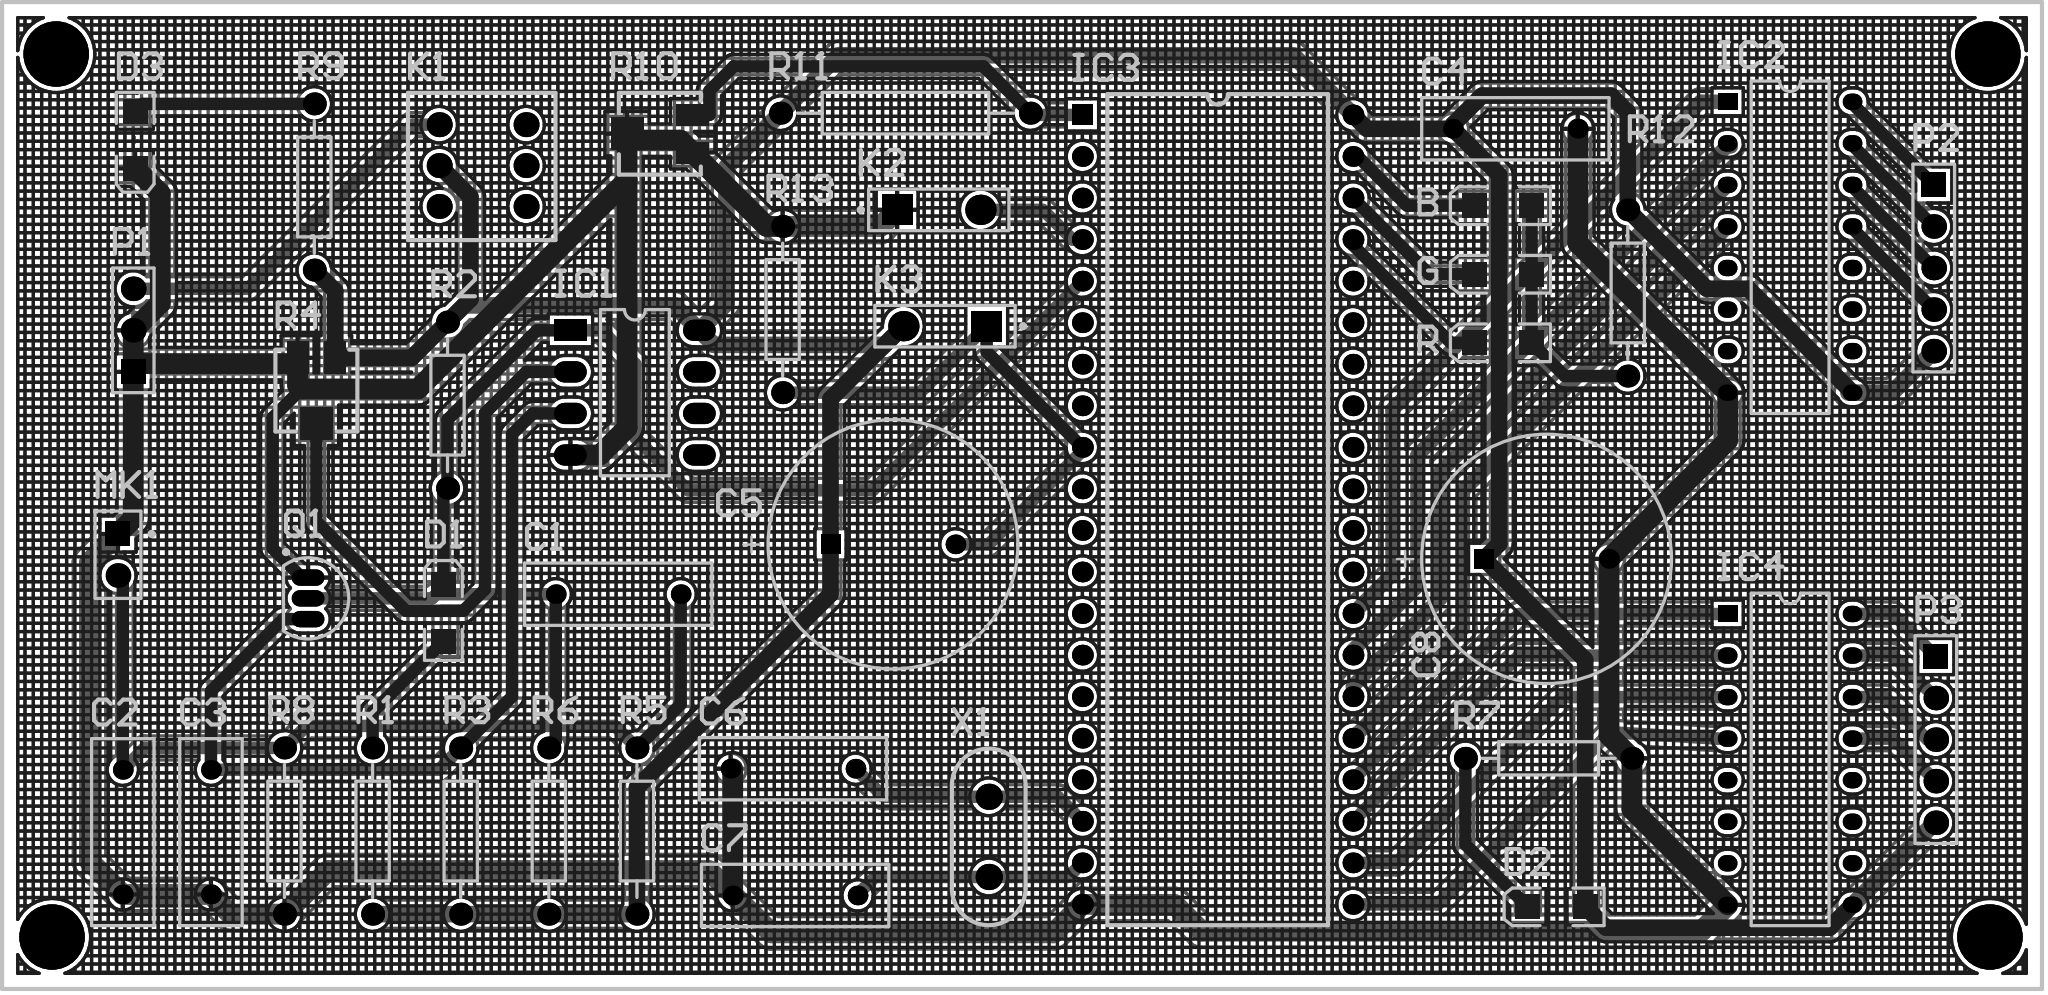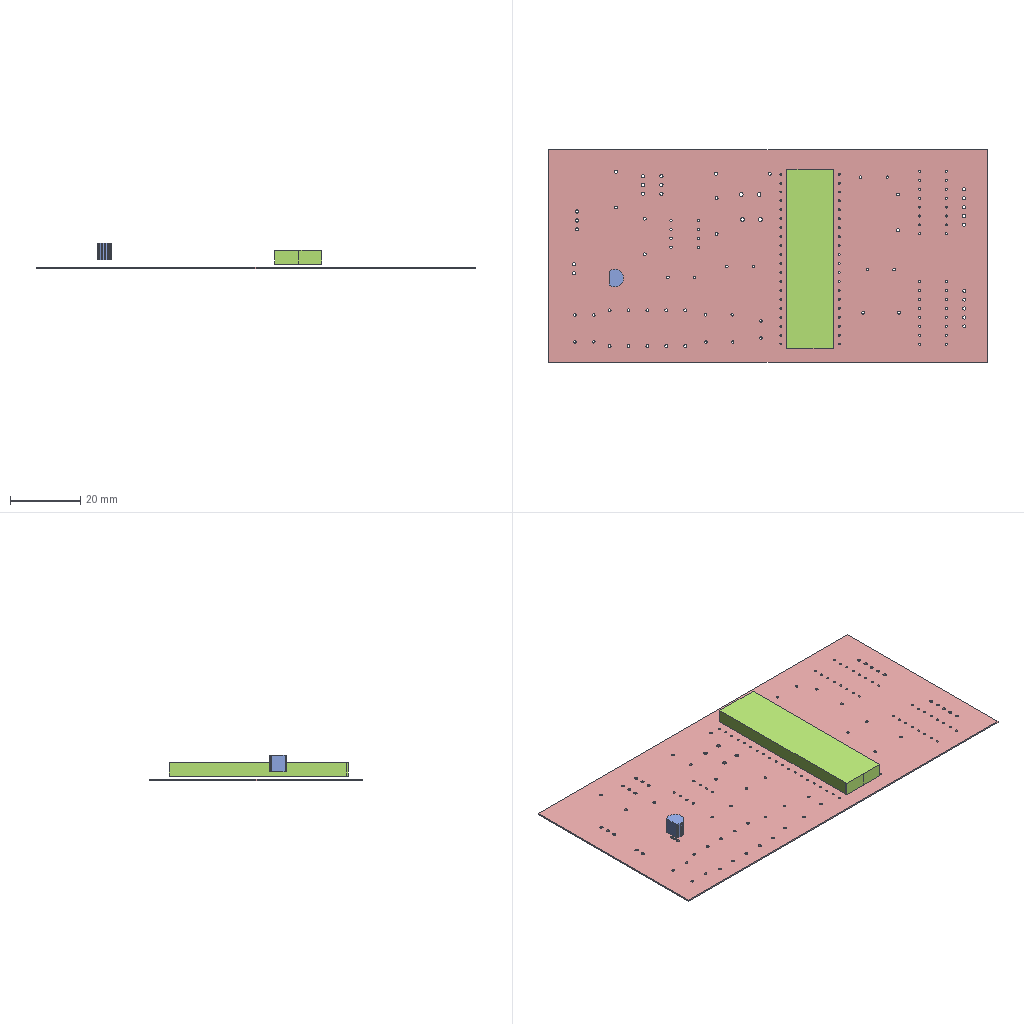Circuit board layout | Altium Designer | box 124.5 x 60.3 x 7.3 mm
Layer stack:
# Altium Designer layer stack of  (unit mm; dielectric type: 0 none, 1 core, 2 prepreg, 3 surface material)
index,name,kind,layer,copper_thickness_mm,dielectric_type,dielectric_thickness_mm,dielectric_material,dielectric_constant
0,Top Paste,other,,,,,,
1,Top Overlay,other,,,,,,
2,Top Solder,dielectric,,,3,0.0102,Solder Resist,3.5
3,Top Layer,copper,Top Layer,0.0356,,,,
4,Dielectric 1,dielectric,,,0,0.32,FR-4,4.8
5,Bottom Layer,copper,Bottom Layer,0.0356,,,,
6,Bottom Solder,dielectric,,,3,0.0102,Solder Resist,3.5
7,Bottom Overlay,other,,,,,,
8,Bottom Paste,other,,,,,,
# drill layer pairs: low layer,high layer
drill_pair,Top Layer,Bottom Layer
Part placement:
Designator,Comment,Layer,Footprint,Center-X(mm),Center-Y(mm),Rotation
X1,Component_1,TopLayer,LC-HC-49S,91.313,60.095,90
R,LED2,TopLayer,3.2X1.6X1.1,122.682,90.297,180
R13,Res2,TopLayer,AXIAL-0.4,78.74,92.329,90
R12,Res2,TopLayer,AXIAL-0.4,130.302,93.345,270
R11,Res Adj2,TopLayer,AXIAL-0.6,86.233,104.334,180
R10,RPot SM,TopLayer,POT4MM-2,71.247,103.077,180
R9,Res2,TopLayer,AXIAL-0.4,50.165,99.822,90
R8,Res2,TopLayer,AXIAL-0.4,48.345,60.452,90
R7,Res2,TopLayer,AXIAL-0.4,125.476,64.897,180
R6,Res2,TopLayer,AXIAL-0.4,64.474,60.452,270
R5,Res2,TopLayer,AXIAL-0.4,69.85,60.452,270
R4,RPot SM,TopLayer,POT4MM-2,50.292,87.376,270
R3,Res2,TopLayer,AXIAL-0.4,59.097,60.452,270
R2,Res2,TopLayer,AXIAL-0.4,58.293,86.487,270
R1,Res2,TopLayer,AXIAL-0.4,53.721,60.452,90
Q1,2N3904,TopLayer,TO-92A,49.784,74.676,180
P3,Header 5,TopLayer,HDR1X5,149.098,66.04,270
P2,Header 5,TopLayer,HDR1X5,148.971,94.869,270
P1,Header 3,TopLayer,HDR1X3,39.116,91.059,90
MK1,Mic2,TopLayer,PIN2,38.186,77.343,270
K3,SW-PB,TopLayer,SPST-2,88.646,91.313,180
K2,SW-PB,TopLayer,SPST-2,88.265,98.425,360
K1,Component_1,TopLayer,自锁开关,60.435,101.132,270
IC4,ULN2003,TopLayer,ULN2003,140.208,64.83,360
IC3,89c51,TopLayer,89c51,105.283,80.097,0
IC2,ULN2003,TopLayer,ULN2003,140.208,96.139,0
IC1,LM393,TopLayer,LM393,69.725,87.249,0
G,LED2,TopLayer,3.2X1.6X1.1,122.682,94.488,180
D3,LED2,TopLayer,3.2X1.6X1.1,39.236,102.704,270
D2,LED2,TopLayer,3.2X1.6X1.1,125.956,55.82,180
D1,LED2,TopLayer,3.2X1.6X1.1,58.039,73.787,90
C8,Cap Pol1,TopLayer,RB7.6-15,125.349,77.089,180
C7,Cap,TopLayer,RAD-0.3,79.502,56.515,180
C6,Cap,TopLayer,RAD-0.3,79.375,64.262,180
C5,Cap Pol1,TopLayer,RB7.6-15,85.471,77.978,180
C4,Cap,TopLayer,RAD-0.3,123.444,103.378,360
C3,Cap,TopLayer,RAD-0.3,43.857,60.385,270
C2,Cap,TopLayer,RAD-0.3,38.481,60.385,270
C1,Cap,TopLayer,RAD-0.3,68.707,74.93,180
B,LED2,TopLayer,3.2X1.6X1.1,122.682,98.679,180
Pad and via stacks:
# Altium Designer via and pad stacks of  (unit mm). Each distinct definition once, with the count of objects using it.
# via: kind,start_layer,end_layer,hole_mm,diameter_mm,mode(0 simple;1 top-mid-bottom;2 full stack),diameter_per_layer,count,example_net
# pad: kind,layer,hole_mm,hole_type(0 round;1 square;2 slot),plating,top_size,top_shape(1 round;2 rect;3 octagon;9 rounded rect),mid_size,bottom_size,mode,footprint,size_per_layer,count,example
pad,Top Layer,0,0,plated,1.5x1.5,2,1.5x1.5,1.5x1.5,0,3.2X1.6X1.1,,12,D1.1
pad,Top Layer,0,0,plated,1.3x2,2,1.3x2,1.3x2,0,POT4MM-2,,4,R4.CCW
pad,Top Layer,0,0,plated,2x2,2,2x2,2x2,0,POT4MM-2,,2,R4.W
pad,Multi-Layer,0.65,0,plated,2x1.3,2,2x1.3,2x1.3,0,LM393,,1,IC1.1
pad,Multi-Layer,0.65,0,plated,2x1.3,1,2x1.3,2x1.3,0,LM393,,7,IC1.2
pad,Multi-Layer,0.6,0,plated,1.2x1,1,1.2x1,1.2x1,0,ULN2003,,30,IC4.9
pad,Multi-Layer,0.6,0,plated,1.2x1,2,1.2x1,1.2x1,0,ULN2003,,2,IC4.1
pad,Multi-Layer,0.9,0,plated,1.5x1.5,2,1.5x1.5,1.5x1.5,0,PIN2,,1,MK1.1
pad,Multi-Layer,0.9,0,plated,1.5x1.5,1,1.5x1.5,1.5x1.5,0,PIN2,,1,MK1.2
pad,Multi-Layer,0.85,0,plated,1.4x1.4,1,1.4x1.4,1.4x1.4,0,AXIAL-0.4,,20,R12.1
pad,Multi-Layer,0.7,0,plated,1.2x1.2,2,1.2x1.2,1.2x1.2,0,RB7.6-15,,2,C5.1
pad,Multi-Layer,0.7,0,plated,1.2x1.2,1,1.2x1.2,1.2x1.2,0,RB7.6-15,,2,C5.2
pad,Multi-Layer,0.85,0,plated,1.4x1.4,1,1.4x1.4,1.4x1.4,0,AXIAL-0.6,,2,R11.2
pad,Multi-Layer,0.9,0,plated,1.5x1.5,2,1.5x1.5,1.5x1.5,0,HDR1X3,,1,P1.1
pad,Multi-Layer,0.9,0,plated,1.5x1.5,1,1.5x1.5,1.5x1.5,0,HDR1X3,,2,P1.2
pad,Multi-Layer,0.7,0,plated,1.2x1.2,1,1.2x1.2,1.2x1.2,0,RAD-0.3,,12,C1.2
pad,Multi-Layer,0.9,0,plated,2x1,1,2x1,2x1,0,TO-92A,,3,Q1.3
pad,Multi-Layer,0.9,0,plated,1.524x1.524,1,1.524x1.524,1.524x1.524,0,\u00D7\u00D4\u00CB\u00F8\u00BF\u00AA\u00B9\u00D8,,6,K1.3
pad,Multi-Layer,0.5588,0,plated,1.27x1.27,2,1.27x1.27,1.27x1.27,0,89c51,,1,IC3.1
pad,Multi-Layer,0.5588,0,plated,1.27x1.27,1,1.27x1.27,1.27x1.27,0,89c51,,39,IC3.2
pad,Multi-Layer,1.1,0,plated,1.85x1.85,2,1.85x1.85,1.85x1.85,0,SPST-2,,2,K2.1
pad,Multi-Layer,1.1,0,plated,1.85x1.85,1,1.85x1.85,1.85x1.85,0,SPST-2,,2,K2.2
pad,Multi-Layer,0.9,0,plated,1.5x1.5,1,1.5x1.5,1.5x1.5,0,HDR1X5,,8,P2.5
pad,Multi-Layer,0.9,0,plated,1.5x1.5,2,1.5x1.5,1.5x1.5,0,HDR1X5,,2,P2.1
pad,Multi-Layer,0.7,0,plated,1.6x1.6,1,1.6x1.6,1.6x1.6,0,LC-HC-49S,,2,X1.1
via,Top Layer,Bottom Layer,3,4,0,,4,
Copper pours:
name,layer,net,type(0 solid;1 hatched;2 none)
Top Layer-No Net,Top Layer,GND,0
Top Layer-No Net,Bottom Layer,GND,0
Design rules, without the lines most boards share:
# Altium Designer design rules of  (exported by Altium Designer, unit mm)
# columns: name | kind | enabled | priority | scope1 | scope2 | descriptor | typed fields (field=value)
GND | 2 | enabled | 1 | InNet('GND') | All | Width Constraint (Min=30mil) (Max=55mil) (Preferred=50mil) (InNet('GND')) |
VCC | 2 | enabled | 2 | InNet('VCC') | All | Width Constraint (Min=30mil) (Max=45mil) (Preferred=40mil) (InNet('VCC')) |
Clearance | 0 | enabled | 1 | All | All | Clearance Constraint (Gap=10mil) (All),(All) | gap=0.254
PlaneConnect | 6 | enabled | 1 | All | All | Power Plane Connect Rule(Relief Connect )(Expansion=20mil) (Conductor Width=10mil) (Air Gap=10mil) (Entries=4) (All) | relief_conductor_width=0.254 relief_entries=4 relief_expansion=0.508
PolygonConnect | 20 | enabled | 1 | All | All | Polygon Connect Rule(Relief Connect )(Conductor Width=10mil) (Relief Angle=90 Angle) (Entries=4) (Air Gap Width=10mil) (All),(All) | connect_style(0=relief,1=direct,2=none)=0 relief_conductor_width=0.254 relief_entries=4
Width | 2 | enabled | 3 | All | All | Width Constraint (Min=20mil) (Max=35mil) (Preferred=30mil) (All) |
RoutingVias | 11 | enabled | 1 | All | All | Routing Via (MinHoleWidth=28mil) (MaxHoleWidth=28mil) (PreferredHoleWidth=28mil) (MinWidth=50mil) (MaxWidth=50mil) (PreferedWidth=50mil) (All) | via_min_hole=0.7112 via_max_hole=0.7112 via_preferred_diameter=1.27 via_preferred_hole=0.7112
PasteMaskExpansion | 14 | enabled | 1 | All | All | Paste Mask Expansion (Expansion =0mil) (All) | expansion=0
SolderMaskExpansion | 13 | enabled | 1 | All | All | Solder Mask Expansion (Expansion =4mil) (All) | expansion=0.1016
HoleSize | 42 | enabled | 1 | All | All | Hole Size Constraint (Min=1mil) (Max=500mil) (All) |
DiffPairsRouting | 51 | enabled | 1 | All | All | Differential Pairs Uncoupled Length using the Gap Constraints (Min=10mil) (Max=10mil) (Prefered=10mil)  and Width Constraints (Min=15mil) (Max=15mil) (Prefered=15mil) (All) |
HoleToHoleClearance | 52 | enabled | 1 | All | All | Hole To Hole Clearance (Gap=10mil) (All),(All) | gap=0.254
MinimumSolderMaskSliver | 53 | enabled | 1 | All | All | Minimum Solder Mask Sliver (Gap=2mil) (All),(All) |
SilkToSolderMaskClearance | 54 | enabled | 1 | IsPad | All | Silk To Solder Mask (Clearance=0mil) (IsPad),(All) |
SilkToSilkClearance | 55 | enabled | 1 | All | All | Silk to Silk (Clearance=2mil) (All),(All) |